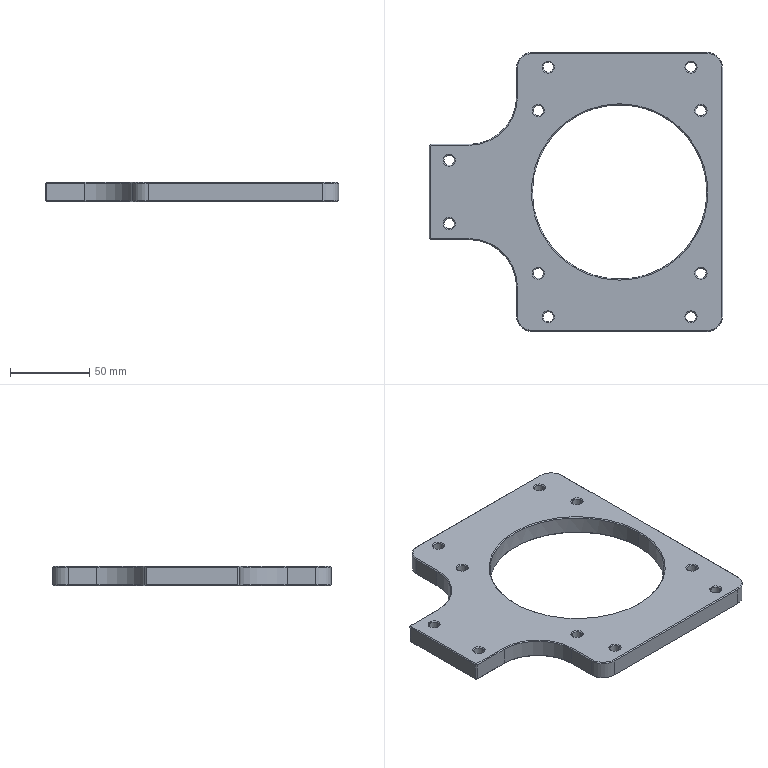Part | SolidWorks | features BaseBody 1 | 1 solid | 116 faces | box 185 x 176 x 12 mm | volume 199285 mm3 | cone 56 | plane 32 | cylinder 28 | commonest cylinder face diameters 6.5 x20 20 x4 60 x2 110 x2